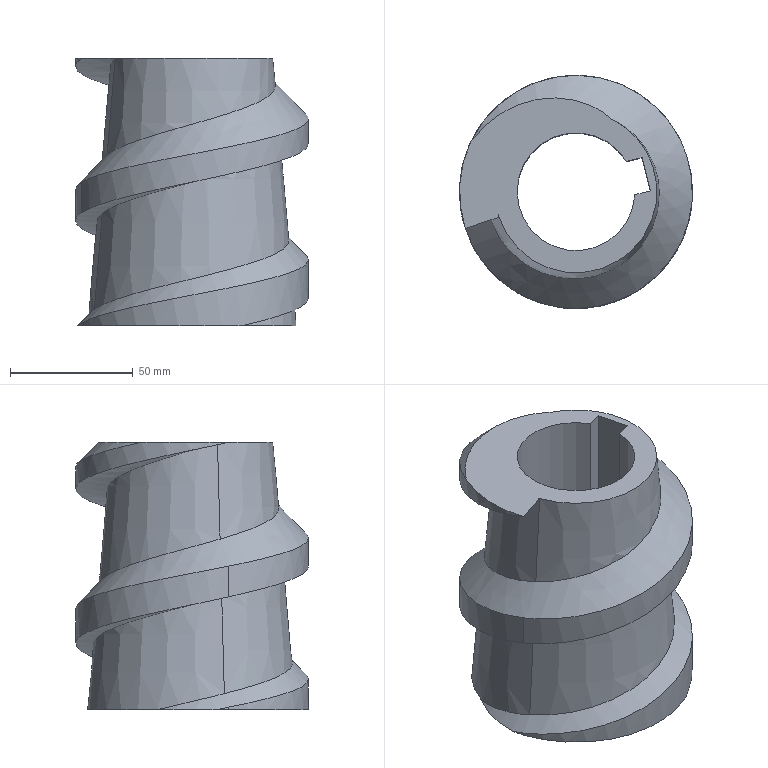Part | SolidWorks | features BaseBody 1, ICE 1, RevCut 1 | 1 solid | 20 faces | box 95.001 x 95.001 x 109 mm | volume 363521 mm3 | cylinder 7 | cone 6 | plane 5 | spline 2 | commonest cylinder face diameters 95 x5 48 x2